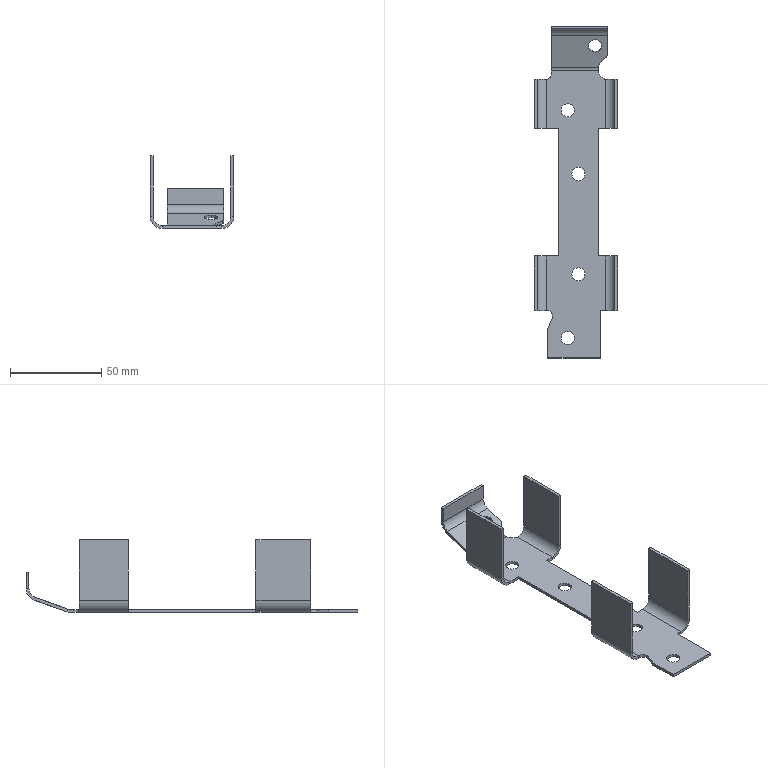Part | SolidWorks | features ICE 2, EdgeFlange 1, FlatPattern 1, SMBaseFlange 1, SheetMetal 1 | 1 solid | 92 faces | box 46 x 182.2 x 40 mm | volume 16049 mm3 | plane 62 | cylinder 26 | spline 4 | commonest cylinder face diameters 7.2 x10 10 x7 13.2 x6 6 x3